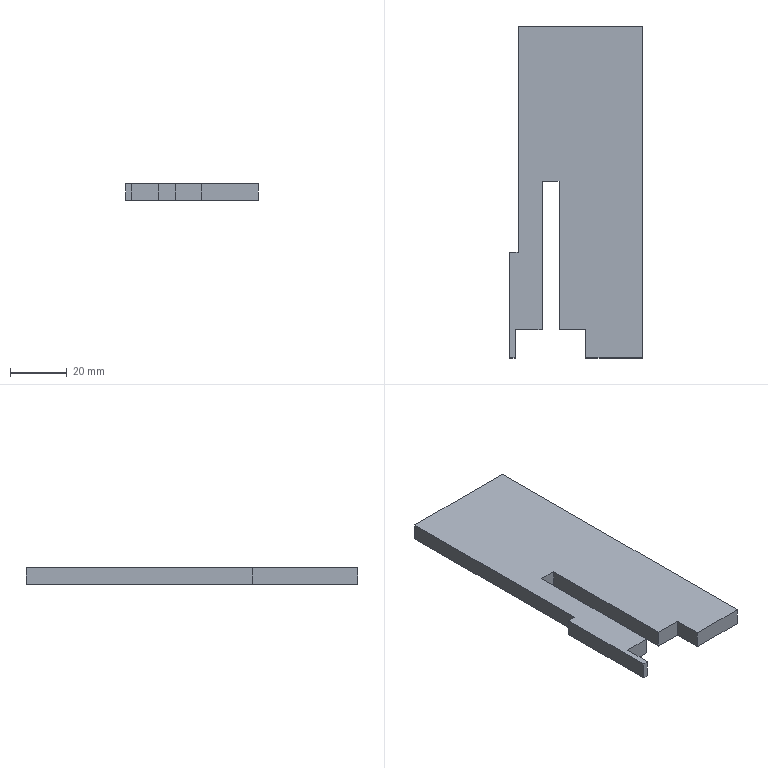Part | SolidWorks | features ICE 2, Extrusion 1 | 1 solid | 16 faces | box 47.002 x 117.5 x 6 mm | volume 28307 mm3 | plane 16
STEP:
#1=CARTESIAN_POINT('',(127.021,-23.445,0.));
#2=VERTEX_POINT('',#1);
#3=CARTESIAN_POINT('',(136.516,-23.453,0.));
#4=VERTEX_POINT('',#3);
#5=CARTESIAN_POINT('',(127.021,-23.445,0.));
#6=DIRECTION('',(1.,-0.0007925,0.));
#7=VECTOR('',#6,1000.);
#8=LINE('',#5,#7);
#9=EDGE_CURVE('',#2,#4,#8,.T.);
#10=ORIENTED_EDGE('',*,*,#9,.T.);
#11=CARTESIAN_POINT('',(136.516,-23.453,6.));
#12=VERTEX_POINT('',#11);
#13=CARTESIAN_POINT('',(136.516,-23.453,6.));
#14=DIRECTION('',(0.,0.,1.));
#15=VECTOR('',#14,1000.);
#16=LINE('',#13,#15);
#17=EDGE_CURVE('',#4,#12,#16,.T.);
#18=ORIENTED_EDGE('',*,*,#17,.T.);
#19=CARTESIAN_POINT('',(127.021,-23.445,6.));
#20=VERTEX_POINT('',#19);
#21=CARTESIAN_POINT('',(127.021,-23.445,6.));
#22=DIRECTION('',(1.,-0.0007925,0.));
#23=VECTOR('',#22,1000.);
#24=LINE('',#21,#23);
#25=EDGE_CURVE('',#20,#12,#24,.T.);
#26=ORIENTED_EDGE('',*,*,#25,.F.);
#27=CARTESIAN_POINT('',(127.021,-23.445,6.));
#28=DIRECTION('',(0.,0.,-1.));
#29=VECTOR('',#28,1000.);
#30=LINE('',#27,#29);
#31=EDGE_CURVE('',#20,#2,#30,.T.);
#32=ORIENTED_EDGE('',*,*,#31,.T.);
#33=EDGE_LOOP('',(#10,#18,#26,#32));
#34=FACE_OUTER_BOUND('',#33,.T.);
#35=CARTESIAN_POINT('',(127.021,-23.445,6.));
#36=DIRECTION('',(0.0007925,1.,0.));
#37=DIRECTION('',(-1.,0.0007925,0.));
#38=AXIS2_PLACEMENT_3D('',#35,#36,#37);
#39=PLANE('',#38);
#40=ADVANCED_FACE('',(#34),#39,.F.);
#41=CARTESIAN_POINT('',(127.013,-33.445,0.));
#42=VERTEX_POINT('',#41);
#43=CARTESIAN_POINT('',(127.013,-33.445,0.));
#44=DIRECTION('',(0.0007925,1.,0.));
#45=VECTOR('',#44,1000.);
#46=LINE('',#43,#45);
#47=EDGE_CURVE('',#42,#2,#46,.T.);
#48=ORIENTED_EDGE('',*,*,#47,.T.);
#49=ORIENTED_EDGE('',*,*,#31,.F.);
#50=CARTESIAN_POINT('',(127.013,-33.445,6.));
#51=VERTEX_POINT('',#50);
#52=CARTESIAN_POINT('',(127.013,-33.445,6.));
#53=DIRECTION('',(0.0007925,1.,0.));
#54=VECTOR('',#53,1000.);
#55=LINE('',#52,#54);
#56=EDGE_CURVE('',#51,#20,#55,.T.);
#57=ORIENTED_EDGE('',*,*,#56,.F.);
#58=CARTESIAN_POINT('',(127.013,-33.445,6.));
#59=DIRECTION('',(0.,0.,-1.));
#60=VECTOR('',#59,1000.);
#61=LINE('',#58,#60);
#62=EDGE_CURVE('',#51,#42,#61,.T.);
#63=ORIENTED_EDGE('',*,*,#62,.T.);
#64=EDGE_LOOP('',(#48,#49,#57,#63));
#65=FACE_OUTER_BOUND('',#64,.T.);
#66=CARTESIAN_POINT('',(127.013,-33.445,6.));
#67=DIRECTION('',(-1.,0.0007925,0.));
#68=DIRECTION('',(-0.0007925,-1.,0.));
#69=AXIS2_PLACEMENT_3D('',#66,#67,#68);
#70=PLANE('',#69);
#71=ADVANCED_FACE('',(#65),#70,.F.);
#72=CARTESIAN_POINT('',(142.516,-23.458,6.));
#73=VERTEX_POINT('',#72);
#74=CARTESIAN_POINT('',(152.022,-23.465,6.));
#75=VERTEX_POINT('',#74);
#76=CARTESIAN_POINT('',(127.021,-23.445,6.));
#77=DIRECTION('',(1.,-0.0007925,0.));
#78=VECTOR('',#77,1000.);
#79=LINE('',#76,#78);
#80=EDGE_CURVE('',#73,#75,#79,.T.);
#81=ORIENTED_EDGE('',*,*,#80,.F.);
#82=CARTESIAN_POINT('',(142.516,-23.458,0.));
#83=VERTEX_POINT('',#82);
#84=CARTESIAN_POINT('',(142.516,-23.458,6.));
#85=DIRECTION('',(0.,0.,-1.));
#86=VECTOR('',#85,1000.);
#87=LINE('',#84,#86);
#88=EDGE_CURVE('',#73,#83,#87,.T.);
#89=ORIENTED_EDGE('',*,*,#88,.T.);
#90=CARTESIAN_POINT('',(152.022,-23.465,0.));
#91=VERTEX_POINT('',#90);
#92=CARTESIAN_POINT('',(127.021,-23.445,0.));
#93=DIRECTION('',(1.,-0.0007925,0.));
#94=VECTOR('',#93,1000.);
#95=LINE('',#92,#94);
#96=EDGE_CURVE('',#83,#91,#95,.T.);
#97=ORIENTED_EDGE('',*,*,#96,.T.);
#98=CARTESIAN_POINT('',(152.022,-23.465,6.));
#99=DIRECTION('',(0.,0.,-1.));
#100=VECTOR('',#99,1000.);
#101=LINE('',#98,#100);
#102=EDGE_CURVE('',#75,#91,#101,.T.);
#103=ORIENTED_EDGE('',*,*,#102,.F.);
#104=EDGE_LOOP('',(#81,#89,#97,#103));
#105=FACE_OUTER_BOUND('',#104,.T.);
#106=CARTESIAN_POINT('',(127.021,-23.445,6.));
#107=DIRECTION('',(0.0007925,1.,0.));
#108=DIRECTION('',(-1.,0.0007925,0.));
#109=AXIS2_PLACEMENT_3D('',#106,#107,#108);
#110=PLANE('',#109);
#111=ADVANCED_FACE('',(#105),#110,.F.);
#112=CARTESIAN_POINT('',(152.015,-33.445,0.));
#113=VERTEX_POINT('',#112);
#114=CARTESIAN_POINT('',(152.022,-23.465,0.));
#115=DIRECTION('',(-0.0007925,-1.,0.));
#116=VECTOR('',#115,1000.);
#117=LINE('',#114,#116);
#118=EDGE_CURVE('',#91,#113,#117,.T.);
#119=ORIENTED_EDGE('',*,*,#118,.T.);
#120=CARTESIAN_POINT('',(152.015,-33.445,6.));
#121=VERTEX_POINT('',#120);
#122=CARTESIAN_POINT('',(152.015,-33.445,6.));
#123=DIRECTION('',(0.,0.,-1.));
#124=VECTOR('',#123,1000.);
#125=LINE('',#122,#124);
#126=EDGE_CURVE('',#121,#113,#125,.T.);
#127=ORIENTED_EDGE('',*,*,#126,.F.);
#128=CARTESIAN_POINT('',(152.022,-23.465,6.));
#129=DIRECTION('',(-0.0007925,-1.,0.));
#130=VECTOR('',#129,1000.);
#131=LINE('',#128,#130);
#132=EDGE_CURVE('',#75,#121,#131,.T.);
#133=ORIENTED_EDGE('',*,*,#132,.F.);
#134=ORIENTED_EDGE('',*,*,#102,.T.);
#135=EDGE_LOOP('',(#119,#127,#133,#134));
#136=FACE_OUTER_BOUND('',#135,.T.);
#137=CARTESIAN_POINT('',(152.022,-23.465,6.));
#138=DIRECTION('',(1.,-0.0007925,0.));
#139=DIRECTION('',(0.0007925,1.,0.));
#140=AXIS2_PLACEMENT_3D('',#137,#138,#139);
#141=PLANE('',#140);
#142=ADVANCED_FACE('',(#136),#141,.F.);
#143=CARTESIAN_POINT('',(172.015,-33.445,0.));
#144=VERTEX_POINT('',#143);
#145=CARTESIAN_POINT('',(152.015,-33.445,0.));
#146=DIRECTION('',(1.,0.,0.));
#147=VECTOR('',#146,1000.);
#148=LINE('',#145,#147);
#149=EDGE_CURVE('',#113,#144,#148,.T.);
#150=ORIENTED_EDGE('',*,*,#149,.T.);
#151=CARTESIAN_POINT('',(172.015,-33.445,6.));
#152=VERTEX_POINT('',#151);
#153=CARTESIAN_POINT('',(172.015,-33.445,6.));
#154=DIRECTION('',(0.,0.,-1.));
#155=VECTOR('',#154,1000.);
#156=LINE('',#153,#155);
#157=EDGE_CURVE('',#152,#144,#156,.T.);
#158=ORIENTED_EDGE('',*,*,#157,.F.);
#159=CARTESIAN_POINT('',(152.015,-33.445,6.));
#160=DIRECTION('',(1.,0.,0.));
#161=VECTOR('',#160,1000.);
#162=LINE('',#159,#161);
#163=EDGE_CURVE('',#121,#152,#162,.T.);
#164=ORIENTED_EDGE('',*,*,#163,.F.);
#165=ORIENTED_EDGE('',*,*,#126,.T.);
#166=EDGE_LOOP('',(#150,#158,#164,#165));
#167=FACE_OUTER_BOUND('',#166,.T.);
#168=CARTESIAN_POINT('',(152.015,-33.445,6.));
#169=DIRECTION('',(0.,1.,0.));
#170=DIRECTION('',(0.,0.,1.));
#171=AXIS2_PLACEMENT_3D('',#168,#169,#170);
#172=PLANE('',#171);
#173=ADVANCED_FACE('',(#167),#172,.F.);
#174=CARTESIAN_POINT('',(172.015,84.055,0.));
#175=VERTEX_POINT('',#174);
#176=CARTESIAN_POINT('',(172.015,-33.445,0.));
#177=DIRECTION('',(0.,1.,0.));
#178=VECTOR('',#177,1000.);
#179=LINE('',#176,#178);
#180=EDGE_CURVE('',#144,#175,#179,.T.);
#181=ORIENTED_EDGE('',*,*,#180,.T.);
#182=CARTESIAN_POINT('',(172.015,84.055,6.));
#183=VERTEX_POINT('',#182);
#184=CARTESIAN_POINT('',(172.015,84.055,6.));
#185=DIRECTION('',(0.,0.,-1.));
#186=VECTOR('',#185,1000.);
#187=LINE('',#184,#186);
#188=EDGE_CURVE('',#183,#175,#187,.T.);
#189=ORIENTED_EDGE('',*,*,#188,.F.);
#190=CARTESIAN_POINT('',(172.015,-33.445,6.));
#191=DIRECTION('',(0.,1.,0.));
#192=VECTOR('',#191,1000.);
#193=LINE('',#190,#192);
#194=EDGE_CURVE('',#152,#183,#193,.T.);
#195=ORIENTED_EDGE('',*,*,#194,.F.);
#196=ORIENTED_EDGE('',*,*,#157,.T.);
#197=EDGE_LOOP('',(#181,#189,#195,#196));
#198=FACE_OUTER_BOUND('',#197,.T.);
#199=CARTESIAN_POINT('',(172.015,-33.445,6.));
#200=DIRECTION('',(-1.,0.,0.));
#201=DIRECTION('',(0.,0.,1.));
#202=AXIS2_PLACEMENT_3D('',#199,#200,#201);
#203=PLANE('',#202);
#204=ADVANCED_FACE('',(#198),#203,.F.);
#205=CARTESIAN_POINT('',(128.013,84.055,0.));
#206=VERTEX_POINT('',#205);
#207=CARTESIAN_POINT('',(172.015,84.055,0.));
#208=DIRECTION('',(-1.,0.,0.));
#209=VECTOR('',#208,1000.);
#210=LINE('',#207,#209);
#211=EDGE_CURVE('',#175,#206,#210,.T.);
#212=ORIENTED_EDGE('',*,*,#211,.T.);
#213=CARTESIAN_POINT('',(128.013,84.055,6.));
#214=VERTEX_POINT('',#213);
#215=CARTESIAN_POINT('',(128.013,84.055,0.));
#216=DIRECTION('',(0.,0.,1.));
#217=VECTOR('',#216,1000.);
#218=LINE('',#215,#217);
#219=EDGE_CURVE('',#206,#214,#218,.T.);
#220=ORIENTED_EDGE('',*,*,#219,.T.);
#221=CARTESIAN_POINT('',(172.015,84.055,6.));
#222=DIRECTION('',(-1.,0.,0.));
#223=VECTOR('',#222,1000.);
#224=LINE('',#221,#223);
#225=EDGE_CURVE('',#183,#214,#224,.T.);
#226=ORIENTED_EDGE('',*,*,#225,.F.);
#227=ORIENTED_EDGE('',*,*,#188,.T.);
#228=EDGE_LOOP('',(#212,#220,#226,#227));
#229=FACE_OUTER_BOUND('',#228,.T.);
#230=CARTESIAN_POINT('',(172.015,84.055,6.));
#231=DIRECTION('',(0.,-1.,0.));
#232=DIRECTION('',(1.,0.,0.));
#233=AXIS2_PLACEMENT_3D('',#230,#231,#232);
#234=PLANE('',#233);
#235=ADVANCED_FACE('',(#229),#234,.F.);
#236=CARTESIAN_POINT('',(125.013,-33.445,6.));
#237=VERTEX_POINT('',#236);
#238=CARTESIAN_POINT('',(127.013,-33.445,6.));
#239=DIRECTION('',(1.,0.,0.));
#240=VECTOR('',#239,1000.);
#241=LINE('',#238,#240);
#242=EDGE_CURVE('',#237,#51,#241,.T.);
#243=ORIENTED_EDGE('',*,*,#242,.F.);
#244=CARTESIAN_POINT('',(125.013,-33.445,0.));
#245=VERTEX_POINT('',#244);
#246=CARTESIAN_POINT('',(125.013,-33.445,6.));
#247=DIRECTION('',(0.,0.,-1.));
#248=VECTOR('',#247,1000.);
#249=LINE('',#246,#248);
#250=EDGE_CURVE('',#237,#245,#249,.T.);
#251=ORIENTED_EDGE('',*,*,#250,.T.);
#252=CARTESIAN_POINT('',(127.013,-33.445,0.));
#253=DIRECTION('',(1.,0.,0.));
#254=VECTOR('',#253,1000.);
#255=LINE('',#252,#254);
#256=EDGE_CURVE('',#245,#42,#255,.T.);
#257=ORIENTED_EDGE('',*,*,#256,.T.);
#258=ORIENTED_EDGE('',*,*,#62,.F.);
#259=EDGE_LOOP('',(#243,#251,#257,#258));
#260=FACE_OUTER_BOUND('',#259,.T.);
#261=CARTESIAN_POINT('',(127.013,-33.445,6.));
#262=DIRECTION('',(0.,1.,0.));
#263=DIRECTION('',(0.,0.,1.));
#264=AXIS2_PLACEMENT_3D('',#261,#262,#263);
#265=PLANE('',#264);
#266=ADVANCED_FACE('',(#260),#265,.F.);
#267=CARTESIAN_POINT('',(125.013,4.055,6.));
#268=VERTEX_POINT('',#267);
#269=CARTESIAN_POINT('',(128.013,4.055,6.));
#270=VERTEX_POINT('',#269);
#271=CARTESIAN_POINT('',(125.013,4.055,6.));
#272=DIRECTION('',(1.,0.,0.));
#273=VECTOR('',#272,1000.);
#274=LINE('',#271,#273);
#275=EDGE_CURVE('',#268,#270,#274,.T.);
#276=ORIENTED_EDGE('',*,*,#275,.F.);
#277=CARTESIAN_POINT('',(125.013,4.055,6.));
#278=DIRECTION('',(0.,1.,0.));
#279=VECTOR('',#278,1000.);
#280=LINE('',#277,#279);
#281=EDGE_CURVE('',#237,#268,#280,.T.);
#282=ORIENTED_EDGE('',*,*,#281,.F.);
#283=ORIENTED_EDGE('',*,*,#242,.T.);
#284=ORIENTED_EDGE('',*,*,#56,.T.);
#285=ORIENTED_EDGE('',*,*,#25,.T.);
#286=CARTESIAN_POINT('',(136.516,29.055,6.));
#287=VERTEX_POINT('',#286);
#288=CARTESIAN_POINT('',(136.516,0.,6.));
#289=DIRECTION('',(0.,1.,0.));
#290=VECTOR('',#289,1000.);
#291=LINE('',#288,#290);
#292=EDGE_CURVE('',#12,#287,#291,.T.);
#293=ORIENTED_EDGE('',*,*,#292,.T.);
#294=CARTESIAN_POINT('',(142.516,29.055,6.));
#295=VERTEX_POINT('',#294);
#296=CARTESIAN_POINT('',(0.,29.055,6.));
#297=DIRECTION('',(1.,0.,0.));
#298=VECTOR('',#297,1000.);
#299=LINE('',#296,#298);
#300=EDGE_CURVE('',#287,#295,#299,.T.);
#301=ORIENTED_EDGE('',*,*,#300,.T.);
#302=CARTESIAN_POINT('',(142.516,0.,6.));
#303=DIRECTION('',(0.,-1.,0.));
#304=VECTOR('',#303,1000.);
#305=LINE('',#302,#304);
#306=EDGE_CURVE('',#295,#73,#305,.T.);
#307=ORIENTED_EDGE('',*,*,#306,.T.);
#308=ORIENTED_EDGE('',*,*,#80,.T.);
#309=ORIENTED_EDGE('',*,*,#132,.T.);
#310=ORIENTED_EDGE('',*,*,#163,.T.);
#311=ORIENTED_EDGE('',*,*,#194,.T.);
#312=ORIENTED_EDGE('',*,*,#225,.T.);
#313=CARTESIAN_POINT('',(128.013,4.055,6.));
#314=DIRECTION('',(0.,1.,0.));
#315=VECTOR('',#314,1000.);
#316=LINE('',#313,#315);
#317=EDGE_CURVE('',#270,#214,#316,.T.);
#318=ORIENTED_EDGE('',*,*,#317,.F.);
#319=EDGE_LOOP('',(#276,#282,#283,#284,#285,#293,#301,#307,#308,#309,#310,#311,#312,#318));
#320=FACE_OUTER_BOUND('',#319,.T.);
#321=CARTESIAN_POINT('',(0.,0.,6.));
#322=DIRECTION('',(0.,0.,-1.));
#323=DIRECTION('',(-1.,0.,0.));
#324=AXIS2_PLACEMENT_3D('',#321,#322,#323);
#325=PLANE('',#324);
#326=ADVANCED_FACE('',(#320),#325,.F.);
#327=CARTESIAN_POINT('',(125.013,4.055,0.));
#328=VERTEX_POINT('',#327);
#329=CARTESIAN_POINT('',(125.013,0.,0.));
#330=DIRECTION('',(0.,-1.,0.));
#331=VECTOR('',#330,1000.);
#332=LINE('',#329,#331);
#333=EDGE_CURVE('',#328,#245,#332,.T.);
#334=ORIENTED_EDGE('',*,*,#333,.F.);
#335=CARTESIAN_POINT('',(128.013,4.055,0.));
#336=VERTEX_POINT('',#335);
#337=CARTESIAN_POINT('',(125.013,4.055,0.));
#338=DIRECTION('',(1.,0.,0.));
#339=VECTOR('',#338,1000.);
#340=LINE('',#337,#339);
#341=EDGE_CURVE('',#328,#336,#340,.T.);
#342=ORIENTED_EDGE('',*,*,#341,.T.);
#343=CARTESIAN_POINT('',(128.013,4.055,0.));
#344=DIRECTION('',(0.,1.,0.));
#345=VECTOR('',#344,1000.);
#346=LINE('',#343,#345);
#347=EDGE_CURVE('',#336,#206,#346,.T.);
#348=ORIENTED_EDGE('',*,*,#347,.T.);
#349=ORIENTED_EDGE('',*,*,#211,.F.);
#350=ORIENTED_EDGE('',*,*,#180,.F.);
#351=ORIENTED_EDGE('',*,*,#149,.F.);
#352=ORIENTED_EDGE('',*,*,#118,.F.);
#353=ORIENTED_EDGE('',*,*,#96,.F.);
#354=CARTESIAN_POINT('',(142.516,29.055,0.));
#355=VERTEX_POINT('',#354);
#356=CARTESIAN_POINT('',(142.516,29.055,0.));
#357=DIRECTION('',(0.,-1.,0.));
#358=VECTOR('',#357,1000.);
#359=LINE('',#356,#358);
#360=EDGE_CURVE('',#355,#83,#359,.T.);
#361=ORIENTED_EDGE('',*,*,#360,.F.);
#362=CARTESIAN_POINT('',(136.516,29.055,0.));
#363=VERTEX_POINT('',#362);
#364=CARTESIAN_POINT('',(142.516,29.055,0.));
#365=DIRECTION('',(1.,0.,0.));
#366=VECTOR('',#365,1000.);
#367=LINE('',#364,#366);
#368=EDGE_CURVE('',#363,#355,#367,.T.);
#369=ORIENTED_EDGE('',*,*,#368,.F.);
#370=CARTESIAN_POINT('',(136.516,0.,0.));
#371=DIRECTION('',(0.,1.,0.));
#372=VECTOR('',#371,1000.);
#373=LINE('',#370,#372);
#374=EDGE_CURVE('',#4,#363,#373,.T.);
#375=ORIENTED_EDGE('',*,*,#374,.F.);
#376=ORIENTED_EDGE('',*,*,#9,.F.);
#377=ORIENTED_EDGE('',*,*,#47,.F.);
#378=ORIENTED_EDGE('',*,*,#256,.F.);
#379=EDGE_LOOP('',(#334,#342,#348,#349,#350,#351,#352,#353,#361,#369,#375,#376,#377,#378));
#380=FACE_OUTER_BOUND('',#379,.T.);
#381=CARTESIAN_POINT('',(0.,0.,0.));
#382=DIRECTION('',(0.,0.,-1.));
#383=DIRECTION('',(-1.,0.,0.));
#384=AXIS2_PLACEMENT_3D('',#381,#382,#383);
#385=PLANE('',#384);
#386=ADVANCED_FACE('',(#380),#385,.T.);
#387=CARTESIAN_POINT('',(136.516,29.055,10.));
#388=DIRECTION('',(0.,0.,-1.));
#389=VECTOR('',#388,1000.);
#390=LINE('',#387,#389);
#391=EDGE_CURVE('',#287,#363,#390,.T.);
#392=ORIENTED_EDGE('',*,*,#391,.T.);
#393=ORIENTED_EDGE('',*,*,#368,.T.);
#394=CARTESIAN_POINT('',(142.516,29.055,10.));
#395=DIRECTION('',(0.,0.,-1.));
#396=VECTOR('',#395,1000.);
#397=LINE('',#394,#396);
#398=EDGE_CURVE('',#295,#355,#397,.T.);
#399=ORIENTED_EDGE('',*,*,#398,.F.);
#400=ORIENTED_EDGE('',*,*,#300,.F.);
#401=EDGE_LOOP('',(#392,#393,#399,#400));
#402=FACE_OUTER_BOUND('',#401,.T.);
#403=CARTESIAN_POINT('',(142.516,29.055,10.));
#404=DIRECTION('',(0.,1.,0.));
#405=DIRECTION('',(0.,0.,1.));
#406=AXIS2_PLACEMENT_3D('',#403,#404,#405);
#407=PLANE('',#406);
#408=ADVANCED_FACE('',(#402),#407,.F.);
#409=ORIENTED_EDGE('',*,*,#374,.T.);
#410=ORIENTED_EDGE('',*,*,#391,.F.);
#411=ORIENTED_EDGE('',*,*,#292,.F.);
#412=ORIENTED_EDGE('',*,*,#17,.F.);
#413=EDGE_LOOP('',(#409,#410,#411,#412));
#414=FACE_OUTER_BOUND('',#413,.T.);
#415=CARTESIAN_POINT('',(136.516,29.055,10.));
#416=DIRECTION('',(-1.,0.,0.));
#417=DIRECTION('',(0.,0.,1.));
#418=AXIS2_PLACEMENT_3D('',#415,#416,#417);
#419=PLANE('',#418);
#420=ADVANCED_FACE('',(#414),#419,.F.);
#421=ORIENTED_EDGE('',*,*,#306,.F.);
#422=ORIENTED_EDGE('',*,*,#398,.T.);
#423=ORIENTED_EDGE('',*,*,#360,.T.);
#424=ORIENTED_EDGE('',*,*,#88,.F.);
#425=EDGE_LOOP('',(#421,#422,#423,#424));
#426=FACE_OUTER_BOUND('',#425,.T.);
#427=CARTESIAN_POINT('',(142.516,29.055,10.));
#428=DIRECTION('',(1.,0.,0.));
#429=DIRECTION('',(0.,0.,-1.));
#430=AXIS2_PLACEMENT_3D('',#427,#428,#429);
#431=PLANE('',#430);
#432=ADVANCED_FACE('',(#426),#431,.F.);
#433=ORIENTED_EDGE('',*,*,#281,.T.);
#434=CARTESIAN_POINT('',(125.013,4.055,0.));
#435=DIRECTION('',(0.,0.,1.));
#436=VECTOR('',#435,1000.);
#437=LINE('',#434,#436);
#438=EDGE_CURVE('',#328,#268,#437,.T.);
#439=ORIENTED_EDGE('',*,*,#438,.F.);
#440=ORIENTED_EDGE('',*,*,#333,.T.);
#441=ORIENTED_EDGE('',*,*,#250,.F.);
#442=EDGE_LOOP('',(#433,#439,#440,#441));
#443=FACE_OUTER_BOUND('',#442,.T.);
#444=CARTESIAN_POINT('',(125.013,4.055,0.));
#445=DIRECTION('',(1.,0.,0.));
#446=DIRECTION('',(0.,0.,-1.));
#447=AXIS2_PLACEMENT_3D('',#444,#445,#446);
#448=PLANE('',#447);
#449=ADVANCED_FACE('',(#443),#448,.F.);
#450=ORIENTED_EDGE('',*,*,#317,.T.);
#451=ORIENTED_EDGE('',*,*,#219,.F.);
#452=ORIENTED_EDGE('',*,*,#347,.F.);
#453=CARTESIAN_POINT('',(128.013,4.055,0.));
#454=DIRECTION('',(0.,0.,1.));
#455=VECTOR('',#454,1000.);
#456=LINE('',#453,#455);
#457=EDGE_CURVE('',#336,#270,#456,.T.);
#458=ORIENTED_EDGE('',*,*,#457,.T.);
#459=EDGE_LOOP('',(#450,#451,#452,#458));
#460=FACE_OUTER_BOUND('',#459,.T.);
#461=CARTESIAN_POINT('',(128.013,4.055,0.));
#462=DIRECTION('',(1.,0.,0.));
#463=DIRECTION('',(0.,0.,-1.));
#464=AXIS2_PLACEMENT_3D('',#461,#462,#463);
#465=PLANE('',#464);
#466=ADVANCED_FACE('',(#460),#465,.F.);
#467=ORIENTED_EDGE('',*,*,#275,.T.);
#468=ORIENTED_EDGE('',*,*,#457,.F.);
#469=ORIENTED_EDGE('',*,*,#341,.F.);
#470=ORIENTED_EDGE('',*,*,#438,.T.);
#471=EDGE_LOOP('',(#467,#468,#469,#470));
#472=FACE_OUTER_BOUND('',#471,.T.);
#473=CARTESIAN_POINT('',(125.013,4.055,0.));
#474=DIRECTION('',(0.,-1.,0.));
#475=DIRECTION('',(0.,0.,-1.));
#476=AXIS2_PLACEMENT_3D('',#473,#474,#475);
#477=PLANE('',#476);
#478=ADVANCED_FACE('',(#472),#477,.F.);
#479=CLOSED_SHELL('',(#40,#71,#111,#142,#173,#204,#235,#266,#326,#386,#408,#420,#432,#449,#466,#478));
#480=MANIFOLD_SOLID_BREP('',#479);
#481=CARTESIAN_POINT('',(0.,0.,0.));
#482=DIRECTION('',(0.,0.,1.));
#483=DIRECTION('',(1.,0.,0.));
#484=AXIS2_PLACEMENT_3D('',#481,#482,#483);
#485=(LENGTH_UNIT()NAMED_UNIT(*)SI_UNIT(.MILLI.,.METRE.));
#486=UNCERTAINTY_MEASURE_WITH_UNIT(LENGTH_MEASURE(0.00001),#485,'','');
#487=(NAMED_UNIT(*)PLANE_ANGLE_UNIT()SI_UNIT($,.RADIAN.));
#488=(NAMED_UNIT(*)SI_UNIT($,.STERADIAN.)SOLID_ANGLE_UNIT());
#489=(GEOMETRIC_REPRESENTATION_CONTEXT(3)GLOBAL_UNCERTAINTY_ASSIGNED_CONTEXT((#486))GLOBAL_UNIT_ASSIGNED_CONTEXT((#485,#487,#488))REPRESENTATION_CONTEXT('',''));
#490=ADVANCED_BREP_SHAPE_REPRESENTATION('',(#480,#484),#489);